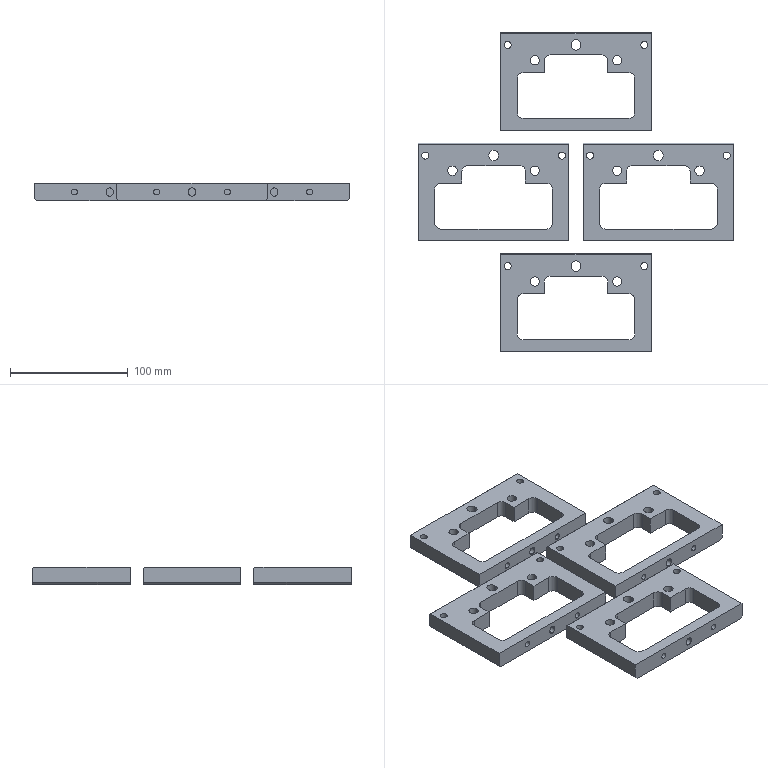NC program | NX | posted with a generic post | part box 268 x 271 x 15 mm
Lines 11348 to 11493 of 34527:
(CAVITY_MILL_COPY_1 , TOOL : D10JING)
N22670 T11 M6
N22672 G54
N22674 G17 G0 G90 X-25.378 Y94.691 B0. C0. S9500 M3
N22676 G43 Z30. H11
N22678 Z-14.
N22680 G94 G1 Z-15. F1000.
N22682 X-26.134 Y96.
N22684 G3 X-27. Y96.5 R1.
N22686 G1 X-45. F1200.
N22688 Y67.5
N22690 X45.
N22692 Y96.5
N22694 X27.
N22696 G2 X22. Y101.5 R5.
N22698 G1 Y111.5
N22700 X-22.
N22702 Y101.5
N22704 G2 X-27. Y96.5 R5.
N22706 G3 X-27.866 Y96. R1.
N22708 G1 X-28.732 Y94.5
N22710 Z-14.
N22712 G0 Z30.
N22714 X-95.378 Y0.691
N22716 Z-14.
N22718 G1 Z-15. F1000.
N22720 X-96.134 Y2.
N22722 G3 X-97. Y2.5 R1.
N22724 G1 X-115. F1200.
N22726 Y-26.5
N22728 X-25.
N22730 Y2.5
N22732 X-43.
N22734 G2 X-48. Y7.5 R5.
N22736 G1 Y17.5
N22738 X-92.
N22740 Y7.5
N22742 G2 X-97. Y2.5 R5.
N22744 G3 X-97.866 Y2. R1.
N22746 G1 X-98.732 Y0.5
N22748 Z-14.
N22750 G0 Z30.
N22752 X-25.378 Y-93.309
N22754 Z-14.
N22756 G1 Z-15. F1000.
N22758 X-26.134 Y-92.
N22760 G3 X-27. Y-91.5 R1.
N22762 G1 X-45. F1200.
N22764 Y-120.5
N22766 X45.
N22768 Y-91.5
N22770 X27.
N22772 G2 X22. Y-86.5 R5.
N22774 G1 Y-76.5
N22776 X-22.
N22778 Y-86.5
N22780 G2 X-27. Y-91.5 R5.
N22782 G3 X-27.866 Y-92. R1.
N22784 G1 X-28.732 Y-93.5
N22786 Z-14.
N22788 G0 Z30.
N22790 X90.191 Y5.878
N22792 Z-14.
N22794 G1 Z-15. F1000.
N22796 X91.5 Y6.634
N22798 G3 X92. Y7.5 R1.
N22800 G1 Y17.5 F1200.
N22802 X48.
N22804 Y7.5
N22806 G2 X43. Y2.5 R5.
N22808 G1 X25.
N22810 Y-26.5
N22812 X115.
N22814 Y2.5
N22816 X97.
N22818 G2 X92. Y7.5 R5.
N22820 G3 X91.5 Y8.366 R1.
N22822 G1 X90. Y9.232
N22824 Z-14.
N22826 G0 Z30.
(ZLEVEL_PROFILE_COPY_1 , TOOL : D10JING)
N22828 X64.558 Y-140.67
N22830 Z-13.95
N22832 G1 Z-14.95 F1000.
N22834 G3 X64. Y-140.5 R1.
N22836 G1 X-64. F1200.
N22838 G2 X-69. Y-135.5 R5.
N22840 G1 Y-52.5
N22842 G2 X-64. Y-47.5 R5.
N22844 G1 X64.
N22846 G2 X69. Y-52.5 R5.
N22848 G1 Y-135.5
N22850 G2 X64. Y-140.5 R5.
N22852 G3 X63.4 Y-140.7 R1.
N22854 G1 Z-13.95
N22856 G0 Z30.
N22858 X-5.442 Y-46.67
N22860 Z-13.95
N22862 G1 Z-14.95 F1000.
N22864 G3 X-6. Y-46.5 R1.
N22866 G1 X-134. F1200.
N22868 G2 X-139. Y-41.5 R5.
N22870 G1 Y41.5
N22872 G2 X-134. Y46.5 R5.
N22874 G1 X-6.
N22876 G2 X-1. Y41.5 R5.
N22878 G1 Y-41.5
N22880 G2 X-6. Y-46.5 R5.
N22882 G3 X-6.6 Y-46.7 R1.
N22884 G1 Z-13.95
N22886 G0 Z30.
N22888 X-64.558 Y140.67
N22890 Z-13.95
N22892 G1 Z-14.95 F1000.
N22894 G3 X-64. Y140.5 R1.
N22896 G1 X64. F1200.
N22898 G2 X69. Y135.5 R5.
N22900 G1 Y52.5
N22902 G2 X64. Y47.5 R5.
N22904 G1 X-64.
N22906 G2 X-69. Y52.5 R5.
N22908 G1 Y135.5
N22910 G2 X-64. Y140.5 R5.
N22912 G3 X-63.4 Y140.7 R1.
N22914 G1 Z-13.95
N22916 G0 Z30.
N22918 X5.442 Y46.67
N22920 Z-13.95
N22922 G1 Z-14.95 F1000.
N22924 G3 X6. Y46.5 R1.
N22926 G1 X134. F1200.
N22928 G2 X139. Y41.5 R5.
N22930 G1 Y-41.5
N22932 G2 X134. Y-46.5 R5.
N22934 G1 X6.
N22936 G2 X1. Y-41.5 R5.
N22938 G1 Y41.5
N22940 G2 X6. Y46.5 R5.
N22942 G3 X6.6 Y46.7 R1.
N22944 G1 Z-13.95
N22946 G0 Z30.
N22948 M5